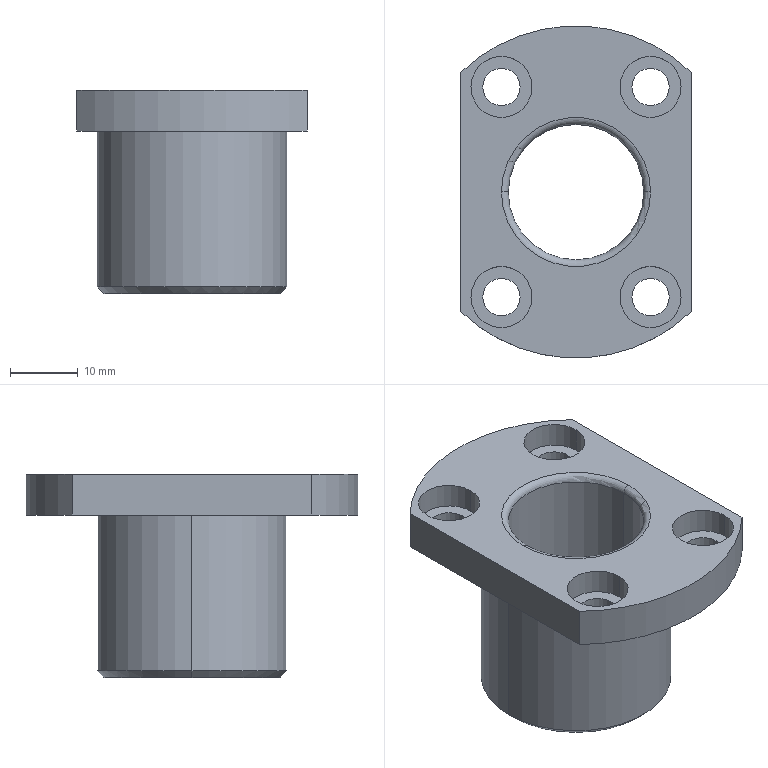Part | STEP file | Guide post flange | 1 solid | 37 faces | box 34 x 49 x 30 mm | volume 13227 mm3 | cylinder 22 | plane 9 | cone 4 | torus 2 | commonest cylinder face diameters 5.5 x8 9 x8 20 x2 28 x2 49 x2
STEP:
#1=CARTESIAN_POINT('',(63.373,-48.431,553.5));
#2=VERTEX_POINT('',#1);
#3=CARTESIAN_POINT('',(37.373,-48.431,553.5));
#4=VERTEX_POINT('',#3);
#5=CARTESIAN_POINT('',(50.373,-48.431,553.5));
#6=DIRECTION('',(0.,0.,-1.));
#7=DIRECTION('',(1.,0.,0.));
#8=AXIS2_PLACEMENT_3D('',#5,#6,#7);
#9=CIRCLE('',#8,13.);
#10=EDGE_CURVE('',#2,#4,#9,.T.);
#11=ORIENTED_EDGE('',*,*,#10,.F.);
#12=CARTESIAN_POINT('',(64.373,-48.431,554.5));
#13=VERTEX_POINT('',#12);
#14=CARTESIAN_POINT('',(63.373,-48.431,553.5));
#15=DIRECTION('',(0.7071,0.,0.7071));
#16=VECTOR('',#15,1000.);
#17=LINE('',#14,#16);
#18=EDGE_CURVE('',#2,#13,#17,.T.);
#19=ORIENTED_EDGE('',*,*,#18,.T.);
#20=CARTESIAN_POINT('',(36.373,-48.431,554.5));
#21=VERTEX_POINT('',#20);
#22=CARTESIAN_POINT('',(50.373,-48.431,554.5));
#23=DIRECTION('',(0.,0.,1.));
#24=DIRECTION('',(1.,0.,0.));
#25=AXIS2_PLACEMENT_3D('',#22,#23,#24);
#26=CIRCLE('',#25,14.);
#27=EDGE_CURVE('',#21,#13,#26,.T.);
#28=ORIENTED_EDGE('',*,*,#27,.F.);
#29=CARTESIAN_POINT('',(37.373,-48.431,553.5));
#30=DIRECTION('',(-0.7071,0.,0.7071));
#31=VECTOR('',#30,1000.);
#32=LINE('',#29,#31);
#33=EDGE_CURVE('',#4,#21,#32,.T.);
#34=ORIENTED_EDGE('',*,*,#33,.F.);
#35=EDGE_LOOP('',(#11,#19,#28,#34));
#36=FACE_OUTER_BOUND('',#35,.T.);
#37=CARTESIAN_POINT('',(50.373,-48.431,553.5));
#38=DIRECTION('',(0.,0.,1.));
#39=DIRECTION('',(-1.,0.,0.));
#40=AXIS2_PLACEMENT_3D('',#37,#38,#39);
#41=CONICAL_SURFACE('',#40,13.,0.7854);
#42=ADVANCED_FACE('',(#36),#41,.T.);
#43=CARTESIAN_POINT('',(40.373,-48.431,554.5));
#44=VERTEX_POINT('',#43);
#45=CARTESIAN_POINT('',(60.373,-48.431,554.5));
#46=VERTEX_POINT('',#45);
#47=CARTESIAN_POINT('',(50.373,-48.431,554.5));
#48=DIRECTION('',(0.,0.,-1.));
#49=DIRECTION('',(1.,0.,0.));
#50=AXIS2_PLACEMENT_3D('',#47,#48,#49);
#51=CIRCLE('',#50,10.);
#52=EDGE_CURVE('',#44,#46,#51,.T.);
#53=ORIENTED_EDGE('',*,*,#52,.F.);
#54=CARTESIAN_POINT('',(39.373,-48.431,553.5));
#55=VERTEX_POINT('',#54);
#56=CARTESIAN_POINT('',(40.373,-48.431,554.5));
#57=DIRECTION('',(-0.7071,0.,-0.7071));
#58=VECTOR('',#57,1000.);
#59=LINE('',#56,#58);
#60=EDGE_CURVE('',#44,#55,#59,.T.);
#61=ORIENTED_EDGE('',*,*,#60,.T.);
#62=CARTESIAN_POINT('',(61.373,-48.431,553.5));
#63=VERTEX_POINT('',#62);
#64=CARTESIAN_POINT('',(50.373,-48.431,553.5));
#65=DIRECTION('',(0.,0.,1.));
#66=DIRECTION('',(1.,0.,0.));
#67=AXIS2_PLACEMENT_3D('',#64,#65,#66);
#68=CIRCLE('',#67,11.);
#69=EDGE_CURVE('',#63,#55,#68,.T.);
#70=ORIENTED_EDGE('',*,*,#69,.F.);
#71=CARTESIAN_POINT('',(60.373,-48.431,554.5));
#72=DIRECTION('',(0.7071,0.,-0.7071));
#73=VECTOR('',#72,1000.);
#74=LINE('',#71,#73);
#75=EDGE_CURVE('',#46,#63,#74,.T.);
#76=ORIENTED_EDGE('',*,*,#75,.F.);
#77=EDGE_LOOP('',(#53,#61,#70,#76));
#78=FACE_OUTER_BOUND('',#77,.T.);
#79=CARTESIAN_POINT('',(50.373,-48.431,554.5));
#80=DIRECTION('',(0.,0.,-1.));
#81=DIRECTION('',(1.,0.,0.));
#82=AXIS2_PLACEMENT_3D('',#79,#80,#81);
#83=CONICAL_SURFACE('',#82,10.,0.7854);
#84=ADVANCED_FACE('',(#78),#83,.F.);
#85=CARTESIAN_POINT('',(61.373,-48.431,583.5));
#86=VERTEX_POINT('',#85);
#87=CARTESIAN_POINT('',(39.373,-48.431,583.5));
#88=VERTEX_POINT('',#87);
#89=CARTESIAN_POINT('',(50.373,-48.431,583.5));
#90=DIRECTION('',(0.,0.,-1.));
#91=DIRECTION('',(-1.,0.,0.));
#92=AXIS2_PLACEMENT_3D('',#89,#90,#91);
#93=CIRCLE('',#92,11.);
#94=EDGE_CURVE('',#86,#88,#93,.T.);
#95=ORIENTED_EDGE('',*,*,#94,.F.);
#96=CARTESIAN_POINT('',(60.373,-48.431,582.5));
#97=VERTEX_POINT('',#96);
#98=CARTESIAN_POINT('',(61.373,-48.431,582.5));
#99=DIRECTION('',(0.,-1.,0.));
#100=DIRECTION('',(1.,0.,0.));
#101=AXIS2_PLACEMENT_3D('',#98,#99,#100);
#102=CIRCLE('',#101,1.);
#103=EDGE_CURVE('',#86,#97,#102,.T.);
#104=ORIENTED_EDGE('',*,*,#103,.T.);
#105=CARTESIAN_POINT('',(40.373,-48.431,582.5));
#106=VERTEX_POINT('',#105);
#107=CARTESIAN_POINT('',(50.373,-48.431,582.5));
#108=DIRECTION('',(0.,0.,1.));
#109=DIRECTION('',(-1.,0.,0.));
#110=AXIS2_PLACEMENT_3D('',#107,#108,#109);
#111=CIRCLE('',#110,10.);
#112=EDGE_CURVE('',#106,#97,#111,.T.);
#113=ORIENTED_EDGE('',*,*,#112,.F.);
#114=CARTESIAN_POINT('',(39.373,-48.431,582.5));
#115=DIRECTION('',(0.,1.,0.));
#116=DIRECTION('',(0.,0.,-1.));
#117=AXIS2_PLACEMENT_3D('',#114,#115,#116);
#118=CIRCLE('',#117,1.);
#119=EDGE_CURVE('',#88,#106,#118,.T.);
#120=ORIENTED_EDGE('',*,*,#119,.F.);
#121=EDGE_LOOP('',(#95,#104,#113,#120));
#122=FACE_OUTER_BOUND('',#121,.T.);
#123=CARTESIAN_POINT('',(50.373,-48.431,582.5));
#124=DIRECTION('',(0.,0.,1.));
#125=DIRECTION('',(-1.,0.,0.));
#126=AXIS2_PLACEMENT_3D('',#123,#124,#125);
#127=TOROIDAL_SURFACE('',#126,11.,1.);
#128=ADVANCED_FACE('',(#122),#127,.T.);
#129=CARTESIAN_POINT('',(43.873,-63.931,579.8));
#130=VERTEX_POINT('',#129);
#131=CARTESIAN_POINT('',(34.873,-63.931,579.8));
#132=VERTEX_POINT('',#131);
#133=CARTESIAN_POINT('',(39.373,-63.931,579.8));
#134=DIRECTION('',(0.,0.,1.));
#135=DIRECTION('',(-1.,0.,0.));
#136=AXIS2_PLACEMENT_3D('',#133,#134,#135);
#137=CIRCLE('',#136,4.5);
#138=EDGE_CURVE('',#130,#132,#137,.T.);
#139=ORIENTED_EDGE('',*,*,#138,.F.);
#140=CARTESIAN_POINT('',(43.873,-63.931,583.5));
#141=VERTEX_POINT('',#140);
#142=CARTESIAN_POINT('',(43.873,-63.931,579.8));
#143=DIRECTION('',(0.,0.,1.));
#144=VECTOR('',#143,1000.);
#145=LINE('',#142,#144);
#146=EDGE_CURVE('',#130,#141,#145,.T.);
#147=ORIENTED_EDGE('',*,*,#146,.T.);
#148=CARTESIAN_POINT('',(34.873,-63.931,583.5));
#149=VERTEX_POINT('',#148);
#150=CARTESIAN_POINT('',(39.373,-63.931,583.5));
#151=DIRECTION('',(0.,0.,1.));
#152=DIRECTION('',(-1.,0.,0.));
#153=AXIS2_PLACEMENT_3D('',#150,#151,#152);
#154=CIRCLE('',#153,4.5);
#155=EDGE_CURVE('',#141,#149,#154,.T.);
#156=ORIENTED_EDGE('',*,*,#155,.T.);
#157=CARTESIAN_POINT('',(34.873,-63.931,579.8));
#158=DIRECTION('',(0.,0.,1.));
#159=VECTOR('',#158,1000.);
#160=LINE('',#157,#159);
#161=EDGE_CURVE('',#132,#149,#160,.T.);
#162=ORIENTED_EDGE('',*,*,#161,.F.);
#163=EDGE_LOOP('',(#139,#147,#156,#162));
#164=FACE_OUTER_BOUND('',#163,.T.);
#165=CARTESIAN_POINT('',(39.373,-63.931,579.8));
#166=DIRECTION('',(0.,0.,1.));
#167=DIRECTION('',(-1.,0.,0.));
#168=AXIS2_PLACEMENT_3D('',#165,#166,#167);
#169=CYLINDRICAL_SURFACE('',#168,4.5);
#170=ADVANCED_FACE('',(#164),#169,.F.);
#171=CARTESIAN_POINT('',(43.873,-32.931,579.8));
#172=VERTEX_POINT('',#171);
#173=CARTESIAN_POINT('',(34.873,-32.931,579.8));
#174=VERTEX_POINT('',#173);
#175=CARTESIAN_POINT('',(39.373,-32.931,579.8));
#176=DIRECTION('',(0.,0.,1.));
#177=DIRECTION('',(-1.,0.,0.));
#178=AXIS2_PLACEMENT_3D('',#175,#176,#177);
#179=CIRCLE('',#178,4.5);
#180=EDGE_CURVE('',#172,#174,#179,.T.);
#181=ORIENTED_EDGE('',*,*,#180,.F.);
#182=CARTESIAN_POINT('',(43.873,-32.931,583.5));
#183=VERTEX_POINT('',#182);
#184=CARTESIAN_POINT('',(43.873,-32.931,579.8));
#185=DIRECTION('',(0.,0.,1.));
#186=VECTOR('',#185,1000.);
#187=LINE('',#184,#186);
#188=EDGE_CURVE('',#172,#183,#187,.T.);
#189=ORIENTED_EDGE('',*,*,#188,.T.);
#190=CARTESIAN_POINT('',(34.873,-32.931,583.5));
#191=VERTEX_POINT('',#190);
#192=CARTESIAN_POINT('',(39.373,-32.931,583.5));
#193=DIRECTION('',(0.,0.,1.));
#194=DIRECTION('',(-1.,0.,0.));
#195=AXIS2_PLACEMENT_3D('',#192,#193,#194);
#196=CIRCLE('',#195,4.5);
#197=EDGE_CURVE('',#183,#191,#196,.T.);
#198=ORIENTED_EDGE('',*,*,#197,.T.);
#199=CARTESIAN_POINT('',(34.873,-32.931,579.8));
#200=DIRECTION('',(0.,0.,1.));
#201=VECTOR('',#200,1000.);
#202=LINE('',#199,#201);
#203=EDGE_CURVE('',#174,#191,#202,.T.);
#204=ORIENTED_EDGE('',*,*,#203,.F.);
#205=EDGE_LOOP('',(#181,#189,#198,#204));
#206=FACE_OUTER_BOUND('',#205,.T.);
#207=CARTESIAN_POINT('',(39.373,-32.931,579.8));
#208=DIRECTION('',(0.,0.,1.));
#209=DIRECTION('',(-1.,0.,0.));
#210=AXIS2_PLACEMENT_3D('',#207,#208,#209);
#211=CYLINDRICAL_SURFACE('',#210,4.5);
#212=ADVANCED_FACE('',(#206),#211,.F.);
#213=CARTESIAN_POINT('',(65.873,-32.931,579.8));
#214=VERTEX_POINT('',#213);
#215=CARTESIAN_POINT('',(56.873,-32.931,579.8));
#216=VERTEX_POINT('',#215);
#217=CARTESIAN_POINT('',(61.373,-32.931,579.8));
#218=DIRECTION('',(0.,0.,1.));
#219=DIRECTION('',(-1.,0.,0.));
#220=AXIS2_PLACEMENT_3D('',#217,#218,#219);
#221=CIRCLE('',#220,4.5);
#222=EDGE_CURVE('',#214,#216,#221,.T.);
#223=ORIENTED_EDGE('',*,*,#222,.F.);
#224=CARTESIAN_POINT('',(65.873,-32.931,583.5));
#225=VERTEX_POINT('',#224);
#226=CARTESIAN_POINT('',(65.873,-32.931,579.8));
#227=DIRECTION('',(0.,0.,1.));
#228=VECTOR('',#227,1000.);
#229=LINE('',#226,#228);
#230=EDGE_CURVE('',#214,#225,#229,.T.);
#231=ORIENTED_EDGE('',*,*,#230,.T.);
#232=CARTESIAN_POINT('',(56.873,-32.931,583.5));
#233=VERTEX_POINT('',#232);
#234=CARTESIAN_POINT('',(61.373,-32.931,583.5));
#235=DIRECTION('',(0.,0.,1.));
#236=DIRECTION('',(-1.,0.,0.));
#237=AXIS2_PLACEMENT_3D('',#234,#235,#236);
#238=CIRCLE('',#237,4.5);
#239=EDGE_CURVE('',#225,#233,#238,.T.);
#240=ORIENTED_EDGE('',*,*,#239,.T.);
#241=CARTESIAN_POINT('',(56.873,-32.931,579.8));
#242=DIRECTION('',(0.,0.,1.));
#243=VECTOR('',#242,1000.);
#244=LINE('',#241,#243);
#245=EDGE_CURVE('',#216,#233,#244,.T.);
#246=ORIENTED_EDGE('',*,*,#245,.F.);
#247=EDGE_LOOP('',(#223,#231,#240,#246));
#248=FACE_OUTER_BOUND('',#247,.T.);
#249=CARTESIAN_POINT('',(61.373,-32.931,579.8));
#250=DIRECTION('',(0.,0.,1.));
#251=DIRECTION('',(-1.,0.,0.));
#252=AXIS2_PLACEMENT_3D('',#249,#250,#251);
#253=CYLINDRICAL_SURFACE('',#252,4.5);
#254=ADVANCED_FACE('',(#248),#253,.F.);
#255=CARTESIAN_POINT('',(65.873,-63.931,579.8));
#256=VERTEX_POINT('',#255);
#257=CARTESIAN_POINT('',(56.873,-63.931,579.8));
#258=VERTEX_POINT('',#257);
#259=CARTESIAN_POINT('',(61.373,-63.931,579.8));
#260=DIRECTION('',(0.,0.,1.));
#261=DIRECTION('',(-1.,0.,0.));
#262=AXIS2_PLACEMENT_3D('',#259,#260,#261);
#263=CIRCLE('',#262,4.5);
#264=EDGE_CURVE('',#256,#258,#263,.T.);
#265=ORIENTED_EDGE('',*,*,#264,.F.);
#266=CARTESIAN_POINT('',(65.873,-63.931,583.5));
#267=VERTEX_POINT('',#266);
#268=CARTESIAN_POINT('',(65.873,-63.931,579.8));
#269=DIRECTION('',(0.,0.,1.));
#270=VECTOR('',#269,1000.);
#271=LINE('',#268,#270);
#272=EDGE_CURVE('',#256,#267,#271,.T.);
#273=ORIENTED_EDGE('',*,*,#272,.T.);
#274=CARTESIAN_POINT('',(56.873,-63.931,583.5));
#275=VERTEX_POINT('',#274);
#276=CARTESIAN_POINT('',(61.373,-63.931,583.5));
#277=DIRECTION('',(0.,0.,1.));
#278=DIRECTION('',(-1.,0.,0.));
#279=AXIS2_PLACEMENT_3D('',#276,#277,#278);
#280=CIRCLE('',#279,4.5);
#281=EDGE_CURVE('',#267,#275,#280,.T.);
#282=ORIENTED_EDGE('',*,*,#281,.T.);
#283=CARTESIAN_POINT('',(56.873,-63.931,579.8));
#284=DIRECTION('',(0.,0.,1.));
#285=VECTOR('',#284,1000.);
#286=LINE('',#283,#285);
#287=EDGE_CURVE('',#258,#275,#286,.T.);
#288=ORIENTED_EDGE('',*,*,#287,.F.);
#289=EDGE_LOOP('',(#265,#273,#282,#288));
#290=FACE_OUTER_BOUND('',#289,.T.);
#291=CARTESIAN_POINT('',(61.373,-63.931,579.8));
#292=DIRECTION('',(0.,0.,1.));
#293=DIRECTION('',(-1.,0.,0.));
#294=AXIS2_PLACEMENT_3D('',#291,#292,#293);
#295=CYLINDRICAL_SURFACE('',#294,4.5);
#296=ADVANCED_FACE('',(#290),#295,.F.);
#297=ORIENTED_EDGE('',*,*,#27,.T.);
#298=CARTESIAN_POINT('',(64.373,-48.431,577.5));
#299=VERTEX_POINT('',#298);
#300=CARTESIAN_POINT('',(64.373,-48.431,553.5));
#301=DIRECTION('',(0.,0.,1.));
#302=VECTOR('',#301,1000.);
#303=LINE('',#300,#302);
#304=EDGE_CURVE('',#13,#299,#303,.T.);
#305=ORIENTED_EDGE('',*,*,#304,.T.);
#306=CARTESIAN_POINT('',(36.373,-48.431,577.5));
#307=VERTEX_POINT('',#306);
#308=CARTESIAN_POINT('',(50.373,-48.431,577.5));
#309=DIRECTION('',(0.,0.,-1.));
#310=DIRECTION('',(-1.,0.,0.));
#311=AXIS2_PLACEMENT_3D('',#308,#309,#310);
#312=CIRCLE('',#311,14.);
#313=EDGE_CURVE('',#299,#307,#312,.T.);
#314=ORIENTED_EDGE('',*,*,#313,.T.);
#315=CARTESIAN_POINT('',(36.373,-48.431,553.5));
#316=DIRECTION('',(0.,0.,1.));
#317=VECTOR('',#316,1000.);
#318=LINE('',#315,#317);
#319=EDGE_CURVE('',#21,#307,#318,.T.);
#320=ORIENTED_EDGE('',*,*,#319,.F.);
#321=EDGE_LOOP('',(#297,#305,#314,#320));
#322=FACE_OUTER_BOUND('',#321,.T.);
#323=CARTESIAN_POINT('',(50.373,-48.431,553.5));
#324=DIRECTION('',(0.,0.,1.));
#325=DIRECTION('',(-1.,0.,0.));
#326=AXIS2_PLACEMENT_3D('',#323,#324,#325);
#327=CYLINDRICAL_SURFACE('',#326,14.);
#328=ADVANCED_FACE('',(#322),#327,.T.);
#329=CARTESIAN_POINT('',(50.373,-48.431,582.5));
#330=DIRECTION('',(0.,0.,1.));
#331=DIRECTION('',(-1.,0.,0.));
#332=AXIS2_PLACEMENT_3D('',#329,#330,#331);
#333=CIRCLE('',#332,10.);
#334=EDGE_CURVE('',#97,#106,#333,.T.);
#335=ORIENTED_EDGE('',*,*,#334,.T.);
#336=CARTESIAN_POINT('',(40.373,-48.431,583.5));
#337=DIRECTION('',(0.,0.,-1.));
#338=VECTOR('',#337,1000.);
#339=LINE('',#336,#338);
#340=EDGE_CURVE('',#106,#44,#339,.T.);
#341=ORIENTED_EDGE('',*,*,#340,.T.);
#342=ORIENTED_EDGE('',*,*,#52,.T.);
#343=CARTESIAN_POINT('',(60.373,-48.431,583.5));
#344=DIRECTION('',(0.,0.,-1.));
#345=VECTOR('',#344,1000.);
#346=LINE('',#343,#345);
#347=EDGE_CURVE('',#97,#46,#346,.T.);
#348=ORIENTED_EDGE('',*,*,#347,.F.);
#349=EDGE_LOOP('',(#335,#341,#342,#348));
#350=FACE_OUTER_BOUND('',#349,.T.);
#351=CARTESIAN_POINT('',(50.373,-48.431,583.5));
#352=DIRECTION('',(0.,0.,-1.));
#353=DIRECTION('',(1.,0.,0.));
#354=AXIS2_PLACEMENT_3D('',#351,#352,#353);
#355=CYLINDRICAL_SURFACE('',#354,10.);
#356=ADVANCED_FACE('',(#350),#355,.F.);
#357=CARTESIAN_POINT('',(64.123,-63.931,579.8));
#358=VERTEX_POINT('',#357);
#359=CARTESIAN_POINT('',(58.623,-63.931,579.8));
#360=VERTEX_POINT('',#359);
#361=CARTESIAN_POINT('',(61.373,-63.931,579.8));
#362=DIRECTION('',(0.,0.,1.));
#363=DIRECTION('',(-1.,0.,0.));
#364=AXIS2_PLACEMENT_3D('',#361,#362,#363);
#365=CIRCLE('',#364,2.75);
#366=EDGE_CURVE('',#358,#360,#365,.T.);
#367=ORIENTED_EDGE('',*,*,#366,.T.);
#368=CARTESIAN_POINT('',(58.623,-63.931,577.5));
#369=VERTEX_POINT('',#368);
#370=CARTESIAN_POINT('',(58.623,-63.931,583.5));
#371=DIRECTION('',(0.,0.,-1.));
#372=VECTOR('',#371,1000.);
#373=LINE('',#370,#372);
#374=EDGE_CURVE('',#360,#369,#373,.T.);
#375=ORIENTED_EDGE('',*,*,#374,.T.);
#376=CARTESIAN_POINT('',(64.123,-63.931,577.5));
#377=VERTEX_POINT('',#376);
#378=CARTESIAN_POINT('',(61.373,-63.931,577.5));
#379=DIRECTION('',(0.,0.,1.));
#380=DIRECTION('',(-1.,0.,0.));
#381=AXIS2_PLACEMENT_3D('',#378,#379,#380);
#382=CIRCLE('',#381,2.75);
#383=EDGE_CURVE('',#377,#369,#382,.T.);
#384=ORIENTED_EDGE('',*,*,#383,.F.);
#385=CARTESIAN_POINT('',(64.123,-63.931,583.5));
#386=DIRECTION('',(0.,0.,-1.));
#387=VECTOR('',#386,1000.);
#388=LINE('',#385,#387);
#389=EDGE_CURVE('',#358,#377,#388,.T.);
#390=ORIENTED_EDGE('',*,*,#389,.F.);
#391=EDGE_LOOP('',(#367,#375,#384,#390));
#392=FACE_OUTER_BOUND('',#391,.T.);
#393=CARTESIAN_POINT('',(61.373,-63.931,583.5));
#394=DIRECTION('',(0.,0.,-1.));
#395=DIRECTION('',(1.,0.,0.));
#396=AXIS2_PLACEMENT_3D('',#393,#394,#395);
#397=CYLINDRICAL_SURFACE('',#396,2.75);
#398=ADVANCED_FACE('',(#392),#397,.F.);
#399=CARTESIAN_POINT('',(64.123,-32.931,579.8));
#400=VERTEX_POINT('',#399);
#401=CARTESIAN_POINT('',(58.623,-32.931,579.8));
#402=VERTEX_POINT('',#401);
#403=CARTESIAN_POINT('',(61.373,-32.931,579.8));
#404=DIRECTION('',(0.,0.,1.));
#405=DIRECTION('',(-1.,0.,0.));
#406=AXIS2_PLACEMENT_3D('',#403,#404,#405);
#407=CIRCLE('',#406,2.75);
#408=EDGE_CURVE('',#400,#402,#407,.T.);
#409=ORIENTED_EDGE('',*,*,#408,.T.);
#410=CARTESIAN_POINT('',(58.623,-32.931,577.5));
#411=VERTEX_POINT('',#410);
#412=CARTESIAN_POINT('',(58.623,-32.931,583.5));
#413=DIRECTION('',(0.,0.,-1.));
#414=VECTOR('',#413,1000.);
#415=LINE('',#412,#414);
#416=EDGE_CURVE('',#402,#411,#415,.T.);
#417=ORIENTED_EDGE('',*,*,#416,.T.);
#418=CARTESIAN_POINT('',(64.123,-32.931,577.5));
#419=VERTEX_POINT('',#418);
#420=CARTESIAN_POINT('',(61.373,-32.931,577.5));
#421=DIRECTION('',(0.,0.,1.));
#422=DIRECTION('',(1.,0.,0.));
#423=AXIS2_PLACEMENT_3D('',#420,#421,#422);
#424=CIRCLE('',#423,2.75);
#425=EDGE_CURVE('',#419,#411,#424,.T.);
#426=ORIENTED_EDGE('',*,*,#425,.F.);
#427=CARTESIAN_POINT('',(64.123,-32.931,583.5));
#428=DIRECTION('',(0.,0.,-1.));
#429=VECTOR('',#428,1000.);
#430=LINE('',#427,#429);
#431=EDGE_CURVE('',#400,#419,#430,.T.);
#432=ORIENTED_EDGE('',*,*,#431,.F.);
#433=EDGE_LOOP('',(#409,#417,#426,#432));
#434=FACE_OUTER_BOUND('',#433,.T.);
#435=CARTESIAN_POINT('',(61.373,-32.931,583.5));
#436=DIRECTION('',(0.,0.,-1.));
#437=DIRECTION('',(1.,0.,0.));
#438=AXIS2_PLACEMENT_3D('',#435,#436,#437);
#439=CYLINDRICAL_SURFACE('',#438,2.75);
#440=ADVANCED_FACE('',(#434),#439,.F.);
#441=CARTESIAN_POINT('',(42.123,-32.931,579.8));
#442=VERTEX_POINT('',#441);
#443=CARTESIAN_POINT('',(36.623,-32.931,579.8));
#444=VERTEX_POINT('',#443);
#445=CARTESIAN_POINT('',(39.373,-32.931,579.8));
#446=DIRECTION('',(0.,0.,1.));
#447=DIRECTION('',(-1.,0.,0.));
#448=AXIS2_PLACEMENT_3D('',#445,#446,#447);
#449=CIRCLE('',#448,2.75);
#450=EDGE_CURVE('',#442,#444,#449,.T.);
#451=ORIENTED_EDGE('',*,*,#450,.T.);
#452=CARTESIAN_POINT('',(36.623,-32.931,577.5));
#453=VERTEX_POINT('',#452);
#454=CARTESIAN_POINT('',(36.623,-32.931,583.5));
#455=DIRECTION('',(0.,0.,-1.));
#456=VECTOR('',#455,1000.);
#457=LINE('',#454,#456);
#458=EDGE_CURVE('',#444,#453,#457,.T.);
#459=ORIENTED_EDGE('',*,*,#458,.T.);
#460=CARTESIAN_POINT('',(42.123,-32.931,577.5));
#461=VERTEX_POINT('',#460);
#462=CARTESIAN_POINT('',(39.373,-32.931,577.5));
#463=DIRECTION('',(0.,0.,1.));
#464=DIRECTION('',(-1.,0.,0.));
#465=AXIS2_PLACEMENT_3D('',#462,#463,#464);
#466=CIRCLE('',#465,2.75);
#467=EDGE_CURVE('',#461,#453,#466,.T.);
#468=ORIENTED_EDGE('',*,*,#467,.F.);
#469=CARTESIAN_POINT('',(42.123,-32.931,583.5));
#470=DIRECTION('',(0.,0.,-1.));
#471=VECTOR('',#470,1000.);
#472=LINE('',#469,#471);
#473=EDGE_CURVE('',#442,#461,#472,.T.);
#474=ORIENTED_EDGE('',*,*,#473,.F.);
#475=EDGE_LOOP('',(#451,#459,#468,#474));
#476=FACE_OUTER_BOUND('',#475,.T.);
#477=CARTESIAN_POINT('',(39.373,-32.931,583.5));
#478=DIRECTION('',(0.,0.,-1.));
#479=DIRECTION('',(1.,0.,0.));
#480=AXIS2_PLACEMENT_3D('',#477,#478,#479);
#481=CYLINDRICAL_SURFACE('',#480,2.75);
#482=ADVANCED_FACE('',(#476),#481,.F.);
#483=CARTESIAN_POINT('',(42.123,-63.931,579.8));
#484=VERTEX_POINT('',#483);
#485=CARTESIAN_POINT('',(36.623,-63.931,579.8));
#486=VERTEX_POINT('',#485);
#487=CARTESIAN_POINT('',(39.373,-63.931,579.8));
#488=DIRECTION('',(0.,0.,1.));
#489=DIRECTION('',(-1.,0.,0.));
#490=AXIS2_PLACEMENT_3D('',#487,#488,#489);
#491=CIRCLE('',#490,2.75);
#492=EDGE_CURVE('',#484,#486,#491,.T.);
#493=ORIENTED_EDGE('',*,*,#492,.T.);
#494=CARTESIAN_POINT('',(36.623,-63.931,577.5));
#495=VERTEX_POINT('',#494);
#496=CARTESIAN_POINT('',(36.623,-63.931,583.5));
#497=DIRECTION('',(0.,0.,-1.));
#498=VECTOR('',#497,1000.);
#499=LINE('',#496,#498);
#500=EDGE_CURVE('',#486,#495,#499,.T.);
#501=ORIENTED_EDGE('',*,*,#500,.T.);
#502=CARTESIAN_POINT('',(42.123,-63.931,577.5));
#503=VERTEX_POINT('',#502);
#504=CARTESIAN_POINT('',(39.373,-63.931,577.5));
#505=DIRECTION('',(0.,0.,1.));
#506=DIRECTION('',(1.,0.,0.));
#507=AXIS2_PLACEMENT_3D('',#504,#505,#506);
#508=CIRCLE('',#507,2.75);
#509=EDGE_CURVE('',#503,#495,#508,.T.);
#510=ORIENTED_EDGE('',*,*,#509,.F.);
#511=CARTESIAN_POINT('',(42.123,-63.931,583.5));
#512=DIRECTION('',(0.,0.,-1.));
#513=VECTOR('',#512,1000.);
#514=LINE('',#511,#513);
#515=EDGE_CURVE('',#484,#503,#514,.T.);
#516=ORIENTED_EDGE('',*,*,#515,.F.);
#517=EDGE_LOOP('',(#493,#501,#510,#516));
#518=FACE_OUTER_BOUND('',#517,.T.);
#519=CARTESIAN_POINT('',(39.373,-63.931,583.5));
#520=DIRECTION('',(0.,0.,-1.));
#521=DIRECTION('',(1.,0.,0.));
#522=AXIS2_PLACEMENT_3D('',#519,#520,#521);
#523=CYLINDRICAL_SURFACE('',#522,2.75);
#524=ADVANCED_FACE('',(#518),#523,.F.);
#525=ORIENTED_EDGE('',*,*,#500,.F.);
#526=CARTESIAN_POINT('',(39.373,-63.931,579.8));
#527=DIRECTION('',(0.,0.,1.));
#528=DIRECTION('',(-1.,0.,0.));
#529=AXIS2_PLACEMENT_3D('',#526,#527,#528);
#530=CIRCLE('',#529,2.75);
#531=EDGE_CURVE('',#486,#484,#530,.T.);
#532=ORIENTED_EDGE('',*,*,#531,.T.);
#533=ORIENTED_EDGE('',*,*,#515,.T.);
#534=CARTESIAN_POINT('',(39.373,-63.931,577.5));
#535=DIRECTION('',(0.,0.,1.));
#536=DIRECTION('',(1.,0.,0.));
#537=AXIS2_PLACEMENT_3D('',#534,#535,#536);
#538=CIRCLE('',#537,2.75);
#539=EDGE_CURVE('',#495,#503,#538,.T.);
#540=ORIENTED_EDGE('',*,*,#539,.F.);
#541=EDGE_LOOP('',(#525,#532,#533,#540));
#542=FACE_OUTER_BOUND('',#541,.T.);
#543=CARTESIAN_POINT('',(39.373,-63.931,583.5));
#544=DIRECTION('',(0.,0.,-1.));
#545=DIRECTION('',(1.,0.,0.));
#546=AXIS2_PLACEMENT_3D('',#543,#544,#545);
#547=CYLINDRICAL_SURFACE('',#546,2.75);
#548=ADVANCED_FACE('',(#542),#547,.F.);
#549=ORIENTED_EDGE('',*,*,#458,.F.);
#550=CARTESIAN_POINT('',(39.373,-32.931,579.8));
#551=DIRECTION('',(0.,0.,1.));
#552=DIRECTION('',(-1.,0.,0.));
#553=AXIS2_PLACEMENT_3D('',#550,#551,#552);
#554=CIRCLE('',#553,2.75);
#555=EDGE_CURVE('',#444,#442,#554,.T.);
#556=ORIENTED_EDGE('',*,*,#555,.T.);
#557=ORIENTED_EDGE('',*,*,#473,.T.);
#558=CARTESIAN_POINT('',(39.373,-32.931,577.5));
#559=DIRECTION('',(0.,0.,1.));
#560=DIRECTION('',(-1.,0.,0.));
#561=AXIS2_PLACEMENT_3D('',#558,#559,#560);
#562=CIRCLE('',#561,2.75);
#563=EDGE_CURVE('',#453,#461,#562,.T.);
#564=ORIENTED_EDGE('',*,*,#563,.F.);
#565=EDGE_LOOP('',(#549,#556,#557,#564));
#566=FACE_OUTER_BOUND('',#565,.T.);
#567=CARTESIAN_POINT('',(39.373,-32.931,583.5));
#568=DIRECTION('',(0.,0.,-1.));
#569=DIRECTION('',(1.,0.,0.));
#570=AXIS2_PLACEMENT_3D('',#567,#568,#569);
#571=CYLINDRICAL_SURFACE('',#570,2.75);
#572=ADVANCED_FACE('',(#566),#571,.F.);
#573=ORIENTED_EDGE('',*,*,#416,.F.);
#574=CARTESIAN_POINT('',(61.373,-32.931,579.8));
#575=DIRECTION('',(0.,0.,1.));
#576=DIRECTION('',(-1.,0.,0.));
#577=AXIS2_PLACEMENT_3D('',#574,#575,#576);
#578=CIRCLE('',#577,2.75);
#579=EDGE_CURVE('',#402,#400,#578,.T.);
#580=ORIENTED_EDGE('',*,*,#579,.T.);
#581=ORIENTED_EDGE('',*,*,#431,.T.);
#582=CARTESIAN_POINT('',(61.373,-32.931,577.5));
#583=DIRECTION('',(0.,0.,1.));
#584=DIRECTION('',(1.,0.,0.));
#585=AXIS2_PLACEMENT_3D('',#582,#583,#584);
#586=CIRCLE('',#585,2.75);
#587=EDGE_CURVE('',#411,#419,#586,.T.);
#588=ORIENTED_EDGE('',*,*,#587,.F.);
#589=EDGE_LOOP('',(#573,#580,#581,#588));
#590=FACE_OUTER_BOUND('',#589,.T.);
#591=CARTESIAN_POINT('',(61.373,-32.931,583.5));
#592=DIRECTION('',(0.,0.,-1.));
#593=DIRECTION('',(1.,0.,0.));
#594=AXIS2_PLACEMENT_3D('',#591,#592,#593);
#595=CYLINDRICAL_SURFACE('',#594,2.75);
#596=ADVANCED_FACE('',(#590),#595,.F.);
#597=ORIENTED_EDGE('',*,*,#374,.F.);
#598=CARTESIAN_POINT('',(61.373,-63.931,579.8));
#599=DIRECTION('',(0.,0.,1.));
#600=DIRECTION('',(-1.,0.,0.));
#601=AXIS2_PLACEMENT_3D('',#598,#599,#600);
#602=CIRCLE('',#601,2.75);
#603=EDGE_CURVE('',#360,#358,#602,.T.);
#604=ORIENTED_EDGE('',*,*,#603,.T.);
#605=ORIENTED_EDGE('',*,*,#389,.T.);
#606=CARTESIAN_POINT('',(61.373,-63.931,577.5));
#607=DIRECTION('',(0.,0.,1.));
#608=DIRECTION('',(-1.,0.,0.));
#609=AXIS2_PLACEMENT_3D('',#606,#607,#608);
#610=CIRCLE('',#609,2.75);
#611=EDGE_CURVE('',#369,#377,#610,.T.);
#612=ORIENTED_EDGE('',*,*,#611,.F.);
#613=EDGE_LOOP('',(#597,#604,#605,#612));
#614=FACE_OUTER_BOUND('',#613,.T.);
#615=CARTESIAN_POINT('',(61.373,-63.931,583.5));
#616=DIRECTION('',(0.,0.,-1.));
#617=DIRECTION('',(1.,0.,0.));
#618=AXIS2_PLACEMENT_3D('',#615,#616,#617);
#619=CYLINDRICAL_SURFACE('',#618,2.75);
#620=ADVANCED_FACE('',(#614),#619,.F.);
#621=CARTESIAN_POINT('',(33.373,-66.073,577.5));
#622=VERTEX_POINT('',#621);
#623=CARTESIAN_POINT('',(67.373,-66.073,577.5));
#624=VERTEX_POINT('',#623);
#625=CARTESIAN_POINT('',(50.373,-48.431,577.5));
#626=DIRECTION('',(0.,0.,1.));
#627=DIRECTION('',(-1.,0.,0.));
#628=AXIS2_PLACEMENT_3D('',#625,#626,#627);
#629=CIRCLE('',#628,24.5);
#630=EDGE_CURVE('',#622,#624,#629,.T.);
#631=ORIENTED_EDGE('',*,*,#630,.F.);
#632=CARTESIAN_POINT('',(33.373,-30.789,577.5));
#633=VERTEX_POINT('',#632);
#634=CARTESIAN_POINT('',(33.373,-66.073,577.5));
#635=DIRECTION('',(0.,-1.,0.));
#636=VECTOR('',#635,1000.);
#637=LINE('',#634,#636);
#638=EDGE_CURVE('',#633,#622,#637,.T.);
#639=ORIENTED_EDGE('',*,*,#638,.F.);
#640=CARTESIAN_POINT('',(67.373,-30.789,577.5));
#641=VERTEX_POINT('',#640);
#642=CARTESIAN_POINT('',(50.373,-48.431,577.5));
#643=DIRECTION('',(0.,0.,1.));
#644=DIRECTION('',(-1.,0.,0.));
#645=AXIS2_PLACEMENT_3D('',#642,#643,#644);
#646=CIRCLE('',#645,24.5);
#647=EDGE_CURVE('',#641,#633,#646,.T.);
#648=ORIENTED_EDGE('',*,*,#647,.F.);
#649=CARTESIAN_POINT('',(67.373,-66.073,577.5));
#650=DIRECTION('',(0.,1.,0.));
#651=VECTOR('',#650,1000.);
#652=LINE('',#649,#651);
#653=EDGE_CURVE('',#624,#641,#652,.T.);
#654=ORIENTED_EDGE('',*,*,#653,.F.);
#655=EDGE_LOOP('',(#631,#639,#648,#654));
#656=FACE_OUTER_BOUND('',#655,.T.);
#657=ORIENTED_EDGE('',*,*,#425,.T.);
#658=ORIENTED_EDGE('',*,*,#587,.T.);
#659=EDGE_LOOP('',(#657,#658));
#660=FACE_BOUND('',#659,.T.);
#661=ORIENTED_EDGE('',*,*,#467,.T.);
#662=ORIENTED_EDGE('',*,*,#563,.T.);
#663=EDGE_LOOP('',(#661,#662));
#664=FACE_BOUND('',#663,.T.);
#665=ORIENTED_EDGE('',*,*,#509,.T.);
#666=ORIENTED_EDGE('',*,*,#539,.T.);
#667=EDGE_LOOP('',(#665,#666));
#668=FACE_BOUND('',#667,.T.);
#669=ORIENTED_EDGE('',*,*,#383,.T.);
#670=ORIENTED_EDGE('',*,*,#611,.T.);
#671=EDGE_LOOP('',(#669,#670));
#672=FACE_BOUND('',#671,.T.);
#673=CARTESIAN_POINT('',(50.373,-48.431,577.5));
#674=DIRECTION('',(0.,0.,-1.));
#675=DIRECTION('',(-1.,0.,0.));
#676=AXIS2_PLACEMENT_3D('',#673,#674,#675);
#677=CIRCLE('',#676,14.);
#678=EDGE_CURVE('',#307,#299,#677,.T.);
#679=ORIENTED_EDGE('',*,*,#678,.F.);
#680=ORIENTED_EDGE('',*,*,#313,.F.);
#681=EDGE_LOOP('',(#679,#680));
#682=FACE_BOUND('',#681,.T.);
#683=CARTESIAN_POINT('',(50.373,-48.431,577.5));
#684=DIRECTION('',(0.,0.,1.));
#685=DIRECTION('',(-1.,0.,0.));
#686=AXIS2_PLACEMENT_3D('',#683,#684,#685);
#687=PLANE('',#686);
#688=ADVANCED_FACE('',(#656,#660,#664,#668,#672,#682),#687,.F.);
#689=CARTESIAN_POINT('',(33.373,-66.073,583.5));
#690=VERTEX_POINT('',#689);
#691=CARTESIAN_POINT('',(67.373,-66.073,583.5));
#692=VERTEX_POINT('',#691);
#693=CARTESIAN_POINT('',(50.373,-48.431,583.5));
#694=DIRECTION('',(0.,0.,1.));
#695=DIRECTION('',(-1.,0.,0.));
#696=AXIS2_PLACEMENT_3D('',#693,#694,#695);
#697=CIRCLE('',#696,24.5);
#698=EDGE_CURVE('',#690,#692,#697,.T.);
#699=ORIENTED_EDGE('',*,*,#698,.T.);
#700=CARTESIAN_POINT('',(67.373,-30.789,583.5));
#701=VERTEX_POINT('',#700);
#702=CARTESIAN_POINT('',(67.373,-66.073,583.5));
#703=DIRECTION('',(0.,1.,0.));
#704=VECTOR('',#703,1000.);
#705=LINE('',#702,#704);
#706=EDGE_CURVE('',#692,#701,#705,.T.);
#707=ORIENTED_EDGE('',*,*,#706,.T.);
#708=CARTESIAN_POINT('',(33.373,-30.789,583.5));
#709=VERTEX_POINT('',#708);
#710=CARTESIAN_POINT('',(50.373,-48.431,583.5));
#711=DIRECTION('',(0.,0.,1.));
#712=DIRECTION('',(-1.,0.,0.));
#713=AXIS2_PLACEMENT_3D('',#710,#711,#712);
#714=CIRCLE('',#713,24.5);
#715=EDGE_CURVE('',#701,#709,#714,.T.);
#716=ORIENTED_EDGE('',*,*,#715,.T.);
#717=CARTESIAN_POINT('',(33.373,-66.073,583.5));
#718=DIRECTION('',(0.,-1.,0.));
#719=VECTOR('',#718,1000.);
#720=LINE('',#717,#719);
#721=EDGE_CURVE('',#709,#690,#720,.T.);
#722=ORIENTED_EDGE('',*,*,#721,.T.);
#723=EDGE_LOOP('',(#699,#707,#716,#722));
#724=FACE_OUTER_BOUND('',#723,.T.);
#725=CARTESIAN_POINT('',(50.373,-48.431,583.5));
#726=DIRECTION('',(0.,0.,-1.));
#727=DIRECTION('',(-1.,0.,0.));
#728=AXIS2_PLACEMENT_3D('',#725,#726,#727);
#729=CIRCLE('',#728,11.);
#730=EDGE_CURVE('',#88,#86,#729,.T.);
#731=ORIENTED_EDGE('',*,*,#730,.T.);
#732=ORIENTED_EDGE('',*,*,#94,.T.);
#733=EDGE_LOOP('',(#731,#732));
#734=FACE_BOUND('',#733,.T.);
#735=CARTESIAN_POINT('',(39.373,-63.931,583.5));
#736=DIRECTION('',(0.,0.,1.));
#737=DIRECTION('',(-1.,0.,0.));
#738=AXIS2_PLACEMENT_3D('',#735,#736,#737);
#739=CIRCLE('',#738,4.5);
#740=EDGE_CURVE('',#149,#141,#739,.T.);
#741=ORIENTED_EDGE('',*,*,#740,.F.);
#742=ORIENTED_EDGE('',*,*,#155,.F.);
#743=EDGE_LOOP('',(#741,#742));
#744=FACE_BOUND('',#743,.T.);
#745=CARTESIAN_POINT('',(39.373,-32.931,583.5));
#746=DIRECTION('',(0.,0.,1.));
#747=DIRECTION('',(-1.,0.,0.));
#748=AXIS2_PLACEMENT_3D('',#745,#746,#747);
#749=CIRCLE('',#748,4.5);
#750=EDGE_CURVE('',#191,#183,#749,.T.);
#751=ORIENTED_EDGE('',*,*,#750,.F.);
#752=ORIENTED_EDGE('',*,*,#197,.F.);
#753=EDGE_LOOP('',(#751,#752));
#754=FACE_BOUND('',#753,.T.);
#755=CARTESIAN_POINT('',(61.373,-32.931,583.5));
#756=DIRECTION('',(0.,0.,1.));
#757=DIRECTION('',(-1.,0.,0.));
#758=AXIS2_PLACEMENT_3D('',#755,#756,#757);
#759=CIRCLE('',#758,4.5);
#760=EDGE_CURVE('',#233,#225,#759,.T.);
#761=ORIENTED_EDGE('',*,*,#760,.F.);
#762=ORIENTED_EDGE('',*,*,#239,.F.);
#763=EDGE_LOOP('',(#761,#762));
#764=FACE_BOUND('',#763,.T.);
#765=CARTESIAN_POINT('',(61.373,-63.931,583.5));
#766=DIRECTION('',(0.,0.,1.));
#767=DIRECTION('',(-1.,0.,0.));
#768=AXIS2_PLACEMENT_3D('',#765,#766,#767);
#769=CIRCLE('',#768,4.5);
#770=EDGE_CURVE('',#275,#267,#769,.T.);
#771=ORIENTED_EDGE('',*,*,#770,.F.);
#772=ORIENTED_EDGE('',*,*,#281,.F.);
#773=EDGE_LOOP('',(#771,#772));
#774=FACE_BOUND('',#773,.T.);
#775=CARTESIAN_POINT('',(50.373,-48.431,583.5));
#776=DIRECTION('',(0.,0.,1.));
#777=DIRECTION('',(-1.,0.,0.));
#778=AXIS2_PLACEMENT_3D('',#775,#776,#777);
#779=PLANE('',#778);
#780=ADVANCED_FACE('',(#724,#734,#744,#754,#764,#774),#779,.T.);
#781=ORIENTED_EDGE('',*,*,#630,.T.);
#782=CARTESIAN_POINT('',(67.373,-66.073,583.5));
#783=DIRECTION('',(0.,0.,-1.));
#784=VECTOR('',#783,1000.);
#785=LINE('',#782,#784);
#786=EDGE_CURVE('',#692,#624,#785,.T.);
#787=ORIENTED_EDGE('',*,*,#786,.F.);
#788=ORIENTED_EDGE('',*,*,#698,.F.);
#789=CARTESIAN_POINT('',(33.373,-66.073,583.5));
#790=DIRECTION('',(0.,0.,-1.));
#791=VECTOR('',#790,1000.);
#792=LINE('',#789,#791);
#793=EDGE_CURVE('',#690,#622,#792,.T.);
#794=ORIENTED_EDGE('',*,*,#793,.T.);
#795=EDGE_LOOP('',(#781,#787,#788,#794));
#796=FACE_OUTER_BOUND('',#795,.T.);
#797=CARTESIAN_POINT('',(50.373,-48.431,583.5));
#798=DIRECTION('',(0.,0.,-1.));
#799=DIRECTION('',(1.,0.,0.));
#800=AXIS2_PLACEMENT_3D('',#797,#798,#799);
#801=CYLINDRICAL_SURFACE('',#800,24.5);
#802=ADVANCED_FACE('',(#796),#801,.T.);
#803=ORIENTED_EDGE('',*,*,#653,.T.);
#804=CARTESIAN_POINT('',(67.373,-30.789,583.5));
#805=DIRECTION('',(0.,0.,-1.));
#806=VECTOR('',#805,1000.);
#807=LINE('',#804,#806);
#808=EDGE_CURVE('',#701,#641,#807,.T.);
#809=ORIENTED_EDGE('',*,*,#808,.F.);
#810=ORIENTED_EDGE('',*,*,#706,.F.);
#811=ORIENTED_EDGE('',*,*,#786,.T.);
#812=EDGE_LOOP('',(#803,#809,#810,#811));
#813=FACE_OUTER_BOUND('',#812,.T.);
#814=CARTESIAN_POINT('',(67.373,-66.073,583.5));
#815=DIRECTION('',(-1.,0.,0.));
#816=DIRECTION('',(0.,-1.,0.));
#817=AXIS2_PLACEMENT_3D('',#814,#815,#816);
#818=PLANE('',#817);
#819=ADVANCED_FACE('',(#813),#818,.F.);
#820=ORIENTED_EDGE('',*,*,#647,.T.);
#821=CARTESIAN_POINT('',(33.373,-30.789,583.5));
#822=DIRECTION('',(0.,0.,-1.));
#823=VECTOR('',#822,1000.);
#824=LINE('',#821,#823);
#825=EDGE_CURVE('',#709,#633,#824,.T.);
#826=ORIENTED_EDGE('',*,*,#825,.F.);
#827=ORIENTED_EDGE('',*,*,#715,.F.);
#828=ORIENTED_EDGE('',*,*,#808,.T.);
#829=EDGE_LOOP('',(#820,#826,#827,#828));
#830=FACE_OUTER_BOUND('',#829,.T.);
#831=CARTESIAN_POINT('',(50.373,-48.431,583.5));
#832=DIRECTION('',(0.,0.,-1.));
#833=DIRECTION('',(1.,0.,0.));
#834=AXIS2_PLACEMENT_3D('',#831,#832,#833);
#835=CYLINDRICAL_SURFACE('',#834,24.5);
#836=ADVANCED_FACE('',(#830),#835,.T.);
#837=ORIENTED_EDGE('',*,*,#638,.T.);
#838=ORIENTED_EDGE('',*,*,#793,.F.);
#839=ORIENTED_EDGE('',*,*,#721,.F.);
#840=ORIENTED_EDGE('',*,*,#825,.T.);
#841=EDGE_LOOP('',(#837,#838,#839,#840));
#842=FACE_OUTER_BOUND('',#841,.T.);
#843=CARTESIAN_POINT('',(33.373,-66.073,583.5));
#844=DIRECTION('',(1.,0.,0.));
#845=DIRECTION('',(0.,-1.,0.));
#846=AXIS2_PLACEMENT_3D('',#843,#844,#845);
#847=PLANE('',#846);
#848=ADVANCED_FACE('',(#842),#847,.F.);
#849=ORIENTED_EDGE('',*,*,#340,.F.);
#850=ORIENTED_EDGE('',*,*,#112,.T.);
#851=ORIENTED_EDGE('',*,*,#347,.T.);
#852=CARTESIAN_POINT('',(50.373,-48.431,554.5));
#853=DIRECTION('',(0.,0.,-1.));
#854=DIRECTION('',(1.,0.,0.));
#855=AXIS2_PLACEMENT_3D('',#852,#853,#854);
#856=CIRCLE('',#855,10.);
#857=EDGE_CURVE('',#46,#44,#856,.T.);
#858=ORIENTED_EDGE('',*,*,#857,.T.);
#859=EDGE_LOOP('',(#849,#850,#851,#858));
#860=FACE_OUTER_BOUND('',#859,.T.);
#861=CARTESIAN_POINT('',(50.373,-48.431,583.5));
#862=DIRECTION('',(0.,0.,-1.));
#863=DIRECTION('',(1.,0.,0.));
#864=AXIS2_PLACEMENT_3D('',#861,#862,#863);
#865=CYLINDRICAL_SURFACE('',#864,10.);
#866=ADVANCED_FACE('',(#860),#865,.F.);
#867=CARTESIAN_POINT('',(50.373,-48.431,553.5));
#868=DIRECTION('',(0.,0.,-1.));
#869=DIRECTION('',(1.,0.,0.));
#870=AXIS2_PLACEMENT_3D('',#867,#868,#869);
#871=CIRCLE('',#870,13.);
#872=EDGE_CURVE('',#4,#2,#871,.T.);
#873=ORIENTED_EDGE('',*,*,#872,.T.);
#874=ORIENTED_EDGE('',*,*,#10,.T.);
#875=EDGE_LOOP('',(#873,#874));
#876=FACE_OUTER_BOUND('',#875,.T.);
#877=ORIENTED_EDGE('',*,*,#69,.T.);
#878=CARTESIAN_POINT('',(50.373,-48.431,553.5));
#879=DIRECTION('',(0.,0.,1.));
#880=DIRECTION('',(1.,0.,0.));
#881=AXIS2_PLACEMENT_3D('',#878,#879,#880);
#882=CIRCLE('',#881,11.);
#883=EDGE_CURVE('',#55,#63,#882,.T.);
#884=ORIENTED_EDGE('',*,*,#883,.T.);
#885=EDGE_LOOP('',(#877,#884));
#886=FACE_BOUND('',#885,.T.);
#887=CARTESIAN_POINT('',(50.373,-48.431,553.5));
#888=DIRECTION('',(0.,0.,-1.));
#889=DIRECTION('',(0.,1.,0.));
#890=AXIS2_PLACEMENT_3D('',#887,#888,#889);
#891=PLANE('',#890);
#892=ADVANCED_FACE('',(#876,#886),#891,.T.);
#893=ORIENTED_EDGE('',*,*,#304,.F.);
#894=CARTESIAN_POINT('',(50.373,-48.431,554.5));
#895=DIRECTION('',(0.,0.,1.));
#896=DIRECTION('',(1.,0.,0.));
#897=AXIS2_PLACEMENT_3D('',#894,#895,#896);
#898=CIRCLE('',#897,14.);
#899=EDGE_CURVE('',#13,#21,#898,.T.);
#900=ORIENTED_EDGE('',*,*,#899,.T.);
#901=ORIENTED_EDGE('',*,*,#319,.T.);
#902=ORIENTED_EDGE('',*,*,#678,.T.);
#903=EDGE_LOOP('',(#893,#900,#901,#902));
#904=FACE_OUTER_BOUND('',#903,.T.);
#905=CARTESIAN_POINT('',(50.373,-48.431,553.5));
#906=DIRECTION('',(0.,0.,1.));
#907=DIRECTION('',(-1.,0.,0.));
#908=AXIS2_PLACEMENT_3D('',#905,#906,#907);
#909=CYLINDRICAL_SURFACE('',#908,14.);
#910=ADVANCED_FACE('',(#904),#909,.T.);
#911=ORIENTED_EDGE('',*,*,#272,.F.);
#912=CARTESIAN_POINT('',(61.373,-63.931,579.8));
#913=DIRECTION('',(0.,0.,1.));
#914=DIRECTION('',(-1.,0.,0.));
#915=AXIS2_PLACEMENT_3D('',#912,#913,#914);
#916=CIRCLE('',#915,4.5);
#917=EDGE_CURVE('',#258,#256,#916,.T.);
#918=ORIENTED_EDGE('',*,*,#917,.F.);
#919=ORIENTED_EDGE('',*,*,#287,.T.);
#920=ORIENTED_EDGE('',*,*,#770,.T.);
#921=EDGE_LOOP('',(#911,#918,#919,#920));
#922=FACE_OUTER_BOUND('',#921,.T.);
#923=CARTESIAN_POINT('',(61.373,-63.931,579.8));
#924=DIRECTION('',(0.,0.,1.));
#925=DIRECTION('',(-1.,0.,0.));
#926=AXIS2_PLACEMENT_3D('',#923,#924,#925);
#927=CYLINDRICAL_SURFACE('',#926,4.5);
#928=ADVANCED_FACE('',(#922),#927,.F.);
#929=ORIENTED_EDGE('',*,*,#917,.T.);
#930=ORIENTED_EDGE('',*,*,#264,.T.);
#931=EDGE_LOOP('',(#929,#930));
#932=FACE_OUTER_BOUND('',#931,.T.);
#933=ORIENTED_EDGE('',*,*,#366,.F.);
#934=ORIENTED_EDGE('',*,*,#603,.F.);
#935=EDGE_LOOP('',(#933,#934));
#936=FACE_BOUND('',#935,.T.);
#937=CARTESIAN_POINT('',(61.373,-63.931,579.8));
#938=DIRECTION('',(0.,0.,1.));
#939=DIRECTION('',(-1.,0.,0.));
#940=AXIS2_PLACEMENT_3D('',#937,#938,#939);
#941=PLANE('',#940);
#942=ADVANCED_FACE('',(#932,#936),#941,.T.);
#943=ORIENTED_EDGE('',*,*,#230,.F.);
#944=CARTESIAN_POINT('',(61.373,-32.931,579.8));
#945=DIRECTION('',(0.,0.,1.));
#946=DIRECTION('',(-1.,0.,0.));
#947=AXIS2_PLACEMENT_3D('',#944,#945,#946);
#948=CIRCLE('',#947,4.5);
#949=EDGE_CURVE('',#216,#214,#948,.T.);
#950=ORIENTED_EDGE('',*,*,#949,.F.);
#951=ORIENTED_EDGE('',*,*,#245,.T.);
#952=ORIENTED_EDGE('',*,*,#760,.T.);
#953=EDGE_LOOP('',(#943,#950,#951,#952));
#954=FACE_OUTER_BOUND('',#953,.T.);
#955=CARTESIAN_POINT('',(61.373,-32.931,579.8));
#956=DIRECTION('',(0.,0.,1.));
#957=DIRECTION('',(-1.,0.,0.));
#958=AXIS2_PLACEMENT_3D('',#955,#956,#957);
#959=CYLINDRICAL_SURFACE('',#958,4.5);
#960=ADVANCED_FACE('',(#954),#959,.F.);
#961=ORIENTED_EDGE('',*,*,#949,.T.);
#962=ORIENTED_EDGE('',*,*,#222,.T.);
#963=EDGE_LOOP('',(#961,#962));
#964=FACE_OUTER_BOUND('',#963,.T.);
#965=ORIENTED_EDGE('',*,*,#408,.F.);
#966=ORIENTED_EDGE('',*,*,#579,.F.);
#967=EDGE_LOOP('',(#965,#966));
#968=FACE_BOUND('',#967,.T.);
#969=CARTESIAN_POINT('',(61.373,-32.931,579.8));
#970=DIRECTION('',(0.,0.,1.));
#971=DIRECTION('',(-1.,0.,0.));
#972=AXIS2_PLACEMENT_3D('',#969,#970,#971);
#973=PLANE('',#972);
#974=ADVANCED_FACE('',(#964,#968),#973,.T.);
#975=ORIENTED_EDGE('',*,*,#188,.F.);
#976=CARTESIAN_POINT('',(39.373,-32.931,579.8));
#977=DIRECTION('',(0.,0.,1.));
#978=DIRECTION('',(-1.,0.,0.));
#979=AXIS2_PLACEMENT_3D('',#976,#977,#978);
#980=CIRCLE('',#979,4.5);
#981=EDGE_CURVE('',#174,#172,#980,.T.);
#982=ORIENTED_EDGE('',*,*,#981,.F.);
#983=ORIENTED_EDGE('',*,*,#203,.T.);
#984=ORIENTED_EDGE('',*,*,#750,.T.);
#985=EDGE_LOOP('',(#975,#982,#983,#984));
#986=FACE_OUTER_BOUND('',#985,.T.);
#987=CARTESIAN_POINT('',(39.373,-32.931,579.8));
#988=DIRECTION('',(0.,0.,1.));
#989=DIRECTION('',(-1.,0.,0.));
#990=AXIS2_PLACEMENT_3D('',#987,#988,#989);
#991=CYLINDRICAL_SURFACE('',#990,4.5);
#992=ADVANCED_FACE('',(#986),#991,.F.);
#993=ORIENTED_EDGE('',*,*,#981,.T.);
#994=ORIENTED_EDGE('',*,*,#180,.T.);
#995=EDGE_LOOP('',(#993,#994));
#996=FACE_OUTER_BOUND('',#995,.T.);
#997=ORIENTED_EDGE('',*,*,#450,.F.);
#998=ORIENTED_EDGE('',*,*,#555,.F.);
#999=EDGE_LOOP('',(#997,#998));
#1000=FACE_BOUND('',#999,.T.);
#1001=CARTESIAN_POINT('',(39.373,-32.931,579.8));
#1002=DIRECTION('',(0.,0.,1.));
#1003=DIRECTION('',(-1.,0.,0.));
#1004=AXIS2_PLACEMENT_3D('',#1001,#1002,#1003);
#1005=PLANE('',#1004);
#1006=ADVANCED_FACE('',(#996,#1000),#1005,.T.);
#1007=ORIENTED_EDGE('',*,*,#146,.F.);
#1008=CARTESIAN_POINT('',(39.373,-63.931,579.8));
#1009=DIRECTION('',(0.,0.,1.));
#1010=DIRECTION('',(-1.,0.,0.));
#1011=AXIS2_PLACEMENT_3D('',#1008,#1009,#1010);
#1012=CIRCLE('',#1011,4.5);
#1013=EDGE_CURVE('',#132,#130,#1012,.T.);
#1014=ORIENTED_EDGE('',*,*,#1013,.F.);
#1015=ORIENTED_EDGE('',*,*,#161,.T.);
#1016=ORIENTED_EDGE('',*,*,#740,.T.);
#1017=EDGE_LOOP('',(#1007,#1014,#1015,#1016));
#1018=FACE_OUTER_BOUND('',#1017,.T.);
#1019=CARTESIAN_POINT('',(39.373,-63.931,579.8));
#1020=DIRECTION('',(0.,0.,1.));
#1021=DIRECTION('',(-1.,0.,0.));
#1022=AXIS2_PLACEMENT_3D('',#1019,#1020,#1021);
#1023=CYLINDRICAL_SURFACE('',#1022,4.5);
#1024=ADVANCED_FACE('',(#1018),#1023,.F.);
#1025=ORIENTED_EDGE('',*,*,#1013,.T.);
#1026=ORIENTED_EDGE('',*,*,#138,.T.);
#1027=EDGE_LOOP('',(#1025,#1026));
#1028=FACE_OUTER_BOUND('',#1027,.T.);
#1029=ORIENTED_EDGE('',*,*,#492,.F.);
#1030=ORIENTED_EDGE('',*,*,#531,.F.);
#1031=EDGE_LOOP('',(#1029,#1030));
#1032=FACE_BOUND('',#1031,.T.);
#1033=CARTESIAN_POINT('',(39.373,-63.931,579.8));
#1034=DIRECTION('',(0.,0.,1.));
#1035=DIRECTION('',(-1.,0.,0.));
#1036=AXIS2_PLACEMENT_3D('',#1033,#1034,#1035);
#1037=PLANE('',#1036);
#1038=ADVANCED_FACE('',(#1028,#1032),#1037,.T.);
#1039=ORIENTED_EDGE('',*,*,#103,.F.);
#1040=ORIENTED_EDGE('',*,*,#730,.F.);
#1041=ORIENTED_EDGE('',*,*,#119,.T.);
#1042=ORIENTED_EDGE('',*,*,#334,.F.);
#1043=EDGE_LOOP('',(#1039,#1040,#1041,#1042));
#1044=FACE_OUTER_BOUND('',#1043,.T.);
#1045=CARTESIAN_POINT('',(50.373,-48.431,582.5));
#1046=DIRECTION('',(0.,0.,1.));
#1047=DIRECTION('',(-1.,0.,0.));
#1048=AXIS2_PLACEMENT_3D('',#1045,#1046,#1047);
#1049=TOROIDAL_SURFACE('',#1048,11.,1.);
#1050=ADVANCED_FACE('',(#1044),#1049,.T.);
#1051=ORIENTED_EDGE('',*,*,#60,.F.);
#1052=ORIENTED_EDGE('',*,*,#857,.F.);
#1053=ORIENTED_EDGE('',*,*,#75,.T.);
#1054=ORIENTED_EDGE('',*,*,#883,.F.);
#1055=EDGE_LOOP('',(#1051,#1052,#1053,#1054));
#1056=FACE_OUTER_BOUND('',#1055,.T.);
#1057=CARTESIAN_POINT('',(50.373,-48.431,554.5));
#1058=DIRECTION('',(0.,0.,-1.));
#1059=DIRECTION('',(1.,0.,0.));
#1060=AXIS2_PLACEMENT_3D('',#1057,#1058,#1059);
#1061=CONICAL_SURFACE('',#1060,10.,0.7854);
#1062=ADVANCED_FACE('',(#1056),#1061,.F.);
#1063=ORIENTED_EDGE('',*,*,#18,.F.);
#1064=ORIENTED_EDGE('',*,*,#872,.F.);
#1065=ORIENTED_EDGE('',*,*,#33,.T.);
#1066=ORIENTED_EDGE('',*,*,#899,.F.);
#1067=EDGE_LOOP('',(#1063,#1064,#1065,#1066));
#1068=FACE_OUTER_BOUND('',#1067,.T.);
#1069=CARTESIAN_POINT('',(50.373,-48.431,553.5));
#1070=DIRECTION('',(0.,0.,1.));
#1071=DIRECTION('',(-1.,0.,0.));
#1072=AXIS2_PLACEMENT_3D('',#1069,#1070,#1071);
#1073=CONICAL_SURFACE('',#1072,13.,0.7854);
#1074=ADVANCED_FACE('',(#1068),#1073,.T.);
#1075=CLOSED_SHELL('',(#42,#84,#128,#170,#212,#254,#296,#328,#356,#398,#440,#482,#524,#548,#572,#596,#620,#688,#780,#802,#819,#836,#848,#866,#892,#910,#928,#942,#960,#974,#992,#1006,#1024,#1038,#1050,#1062,#1074));
#1076=MANIFOLD_SOLID_BREP('',#1075);
#1077=CARTESIAN_POINT('',(0.,0.,0.));
#1078=DIRECTION('',(0.,0.,1.));
#1079=DIRECTION('',(1.,0.,0.));
#1080=AXIS2_PLACEMENT_3D('',#1077,#1078,#1079);
#1081=(LENGTH_UNIT()NAMED_UNIT(*)SI_UNIT(.MILLI.,.METRE.));
#1082=UNCERTAINTY_MEASURE_WITH_UNIT(LENGTH_MEASURE(0.00001),#1081,'','');
#1083=(NAMED_UNIT(*)PLANE_ANGLE_UNIT()SI_UNIT($,.RADIAN.));
#1084=(NAMED_UNIT(*)SI_UNIT($,.STERADIAN.)SOLID_ANGLE_UNIT());
#1085=(GEOMETRIC_REPRESENTATION_CONTEXT(3)GLOBAL_UNCERTAINTY_ASSIGNED_CONTEXT((#1082))GLOBAL_UNIT_ASSIGNED_CONTEXT((#1081,#1083,#1084))REPRESENTATION_CONTEXT('',''));
#1086=ADVANCED_BREP_SHAPE_REPRESENTATION('',(#1076,#1080),#1085);